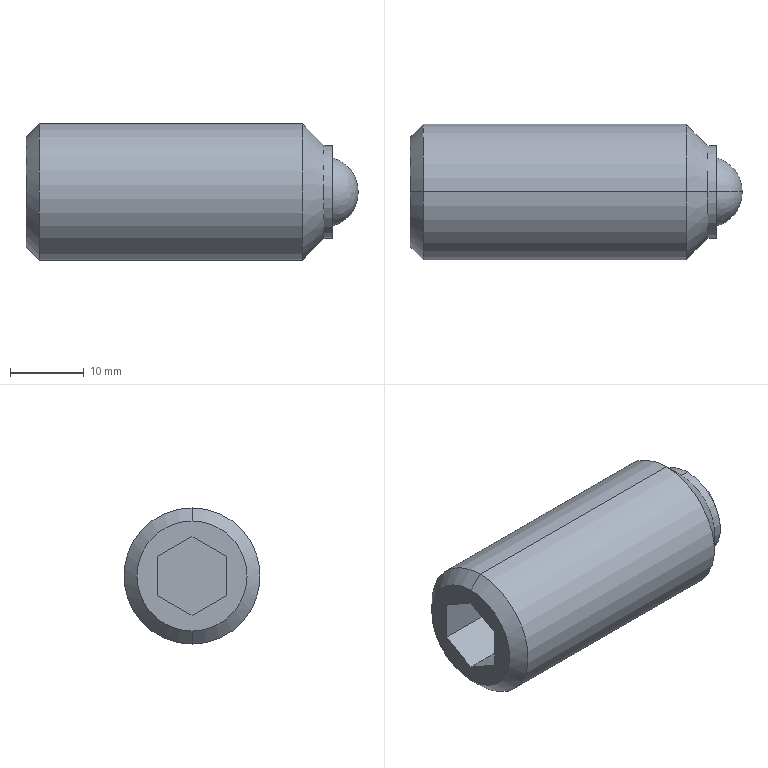Part | SolidWorks | features BaseBody 1 | 1 solid | 19 faces | box 45.002 x 18.462 x 18.462 mm | volume 10278 mm3 | plane 9 | cylinder 4 | cone 4 | spline 2 | commonest cylinder face diameters 12.614 x2 18.462 x2
STEP:
#1=CARTESIAN_POINT('',(0.09191,323.346,152.692));
#2=VERTEX_POINT('',#1);
#3=CARTESIAN_POINT('',(0.09191,323.346,134.231));
#4=VERTEX_POINT('',#3);
#5=CARTESIAN_POINT('',(0.09191,323.346,143.462));
#6=DIRECTION('',(-1.,0.,0.));
#7=DIRECTION('',(0.,0.,1.));
#8=AXIS2_PLACEMENT_3D('',#5,#6,#7);
#9=CIRCLE('',#8,9.231);
#10=EDGE_CURVE('',#2,#4,#9,.T.);
#11=ORIENTED_EDGE('',*,*,#10,.T.);
#12=CARTESIAN_POINT('',(-35.599,323.346,134.231));
#13=VERTEX_POINT('',#12);
#14=CARTESIAN_POINT('',(7.631,323.346,134.231));
#15=DIRECTION('',(-1.,0.,0.));
#16=VECTOR('',#15,1000.);
#17=LINE('',#14,#16);
#18=EDGE_CURVE('',#4,#13,#17,.T.);
#19=ORIENTED_EDGE('',*,*,#18,.T.);
#20=CARTESIAN_POINT('',(-35.599,323.346,152.692));
#21=VERTEX_POINT('',#20);
#22=CARTESIAN_POINT('',(-35.599,323.346,143.462));
#23=DIRECTION('',(1.,0.,0.));
#24=DIRECTION('',(0.,0.,1.));
#25=AXIS2_PLACEMENT_3D('',#22,#23,#24);
#26=CIRCLE('',#25,9.231);
#27=EDGE_CURVE('',#13,#21,#26,.T.);
#28=ORIENTED_EDGE('',*,*,#27,.T.);
#29=CARTESIAN_POINT('',(7.631,323.346,152.692));
#30=DIRECTION('',(-1.,0.,0.));
#31=VECTOR('',#30,1000.);
#32=LINE('',#29,#31);
#33=EDGE_CURVE('',#2,#21,#32,.T.);
#34=ORIENTED_EDGE('',*,*,#33,.F.);
#35=EDGE_LOOP('',(#11,#19,#28,#34));
#36=FACE_OUTER_BOUND('',#35,.T.);
#37=CARTESIAN_POINT('',(7.631,323.346,143.462));
#38=DIRECTION('',(-1.,0.,0.));
#39=DIRECTION('',(0.,0.,1.));
#40=AXIS2_PLACEMENT_3D('',#37,#38,#39);
#41=CYLINDRICAL_SURFACE('',#40,9.231);
#42=ADVANCED_FACE('',(#36),#41,.T.);
#43=CARTESIAN_POINT('',(-37.369,323.346,136.001));
#44=VERTEX_POINT('',#43);
#45=CARTESIAN_POINT('',(-37.369,323.346,150.922));
#46=VERTEX_POINT('',#45);
#47=CARTESIAN_POINT('',(-37.369,323.346,143.462));
#48=DIRECTION('',(1.,0.,0.));
#49=DIRECTION('',(0.,0.,-1.));
#50=AXIS2_PLACEMENT_3D('',#47,#48,#49);
#51=CIRCLE('',#50,7.461);
#52=EDGE_CURVE('',#44,#46,#51,.T.);
#53=ORIENTED_EDGE('',*,*,#52,.T.);
#54=CARTESIAN_POINT('',(-35.599,323.346,152.692));
#55=DIRECTION('',(0.7071,0.,0.7071));
#56=VECTOR('',#55,1000.);
#57=LINE('',#54,#56);
#58=EDGE_CURVE('',#46,#21,#57,.T.);
#59=ORIENTED_EDGE('',*,*,#58,.T.);
#60=ORIENTED_EDGE('',*,*,#27,.F.);
#61=CARTESIAN_POINT('',(-35.599,323.346,134.231));
#62=DIRECTION('',(0.7071,0.,-0.7071));
#63=VECTOR('',#62,1000.);
#64=LINE('',#61,#63);
#65=EDGE_CURVE('',#44,#13,#64,.T.);
#66=ORIENTED_EDGE('',*,*,#65,.F.);
#67=EDGE_LOOP('',(#53,#59,#60,#66));
#68=FACE_OUTER_BOUND('',#67,.T.);
#69=CARTESIAN_POINT('',(-35.599,323.346,143.462));
#70=DIRECTION('',(1.,0.,0.));
#71=DIRECTION('',(0.,0.,-1.));
#72=AXIS2_PLACEMENT_3D('',#69,#70,#71);
#73=CONICAL_SURFACE('',#72,9.231,0.7854);
#74=ADVANCED_FACE('',(#68),#73,.T.);
#75=CARTESIAN_POINT('',(3.016,323.346,149.768));
#76=VERTEX_POINT('',#75);
#77=CARTESIAN_POINT('',(3.016,323.346,137.155));
#78=VERTEX_POINT('',#77);
#79=CARTESIAN_POINT('',(3.016,323.346,143.462));
#80=DIRECTION('',(-1.,0.,0.));
#81=DIRECTION('',(0.,-1.,0.));
#82=AXIS2_PLACEMENT_3D('',#79,#80,#81);
#83=CIRCLE('',#82,6.307);
#84=EDGE_CURVE('',#76,#78,#83,.T.);
#85=ORIENTED_EDGE('',*,*,#84,.T.);
#86=CARTESIAN_POINT('',(0.09191,323.346,134.231));
#87=DIRECTION('',(-0.7071,0.,-0.7071));
#88=VECTOR('',#87,1000.);
#89=LINE('',#86,#88);
#90=EDGE_CURVE('',#78,#4,#89,.T.);
#91=ORIENTED_EDGE('',*,*,#90,.T.);
#92=ORIENTED_EDGE('',*,*,#10,.F.);
#93=CARTESIAN_POINT('',(0.09191,323.346,152.692));
#94=DIRECTION('',(-0.7071,0.,0.7071));
#95=VECTOR('',#94,1000.);
#96=LINE('',#93,#95);
#97=EDGE_CURVE('',#76,#2,#96,.T.);
#98=ORIENTED_EDGE('',*,*,#97,.F.);
#99=EDGE_LOOP('',(#85,#91,#92,#98));
#100=FACE_OUTER_BOUND('',#99,.T.);
#101=CARTESIAN_POINT('',(0.09191,323.346,143.462));
#102=DIRECTION('',(-1.,0.,0.));
#103=DIRECTION('',(0.,0.,1.));
#104=AXIS2_PLACEMENT_3D('',#101,#102,#103);
#105=CONICAL_SURFACE('',#104,9.231,0.7854);
#106=ADVANCED_FACE('',(#100),#105,.T.);
#107=CARTESIAN_POINT('',(4.17,323.346,149.768));
#108=VERTEX_POINT('',#107);
#109=CARTESIAN_POINT('',(4.17,323.346,137.155));
#110=VERTEX_POINT('',#109);
#111=CARTESIAN_POINT('',(4.17,323.346,143.462));
#112=DIRECTION('',(-1.,0.,0.));
#113=DIRECTION('',(0.,0.,1.));
#114=AXIS2_PLACEMENT_3D('',#111,#112,#113);
#115=CIRCLE('',#114,6.307);
#116=EDGE_CURVE('',#108,#110,#115,.T.);
#117=ORIENTED_EDGE('',*,*,#116,.T.);
#118=CARTESIAN_POINT('',(7.631,323.346,137.155));
#119=DIRECTION('',(-1.,0.,0.));
#120=VECTOR('',#119,1000.);
#121=LINE('',#118,#120);
#122=EDGE_CURVE('',#110,#78,#121,.T.);
#123=ORIENTED_EDGE('',*,*,#122,.T.);
#124=ORIENTED_EDGE('',*,*,#84,.F.);
#125=CARTESIAN_POINT('',(7.631,323.346,149.768));
#126=DIRECTION('',(-1.,0.,0.));
#127=VECTOR('',#126,1000.);
#128=LINE('',#125,#127);
#129=EDGE_CURVE('',#108,#76,#128,.T.);
#130=ORIENTED_EDGE('',*,*,#129,.F.);
#131=EDGE_LOOP('',(#117,#123,#124,#130));
#132=FACE_OUTER_BOUND('',#131,.T.);
#133=CARTESIAN_POINT('',(7.631,323.346,143.462));
#134=DIRECTION('',(-1.,0.,0.));
#135=DIRECTION('',(0.,0.,1.));
#136=AXIS2_PLACEMENT_3D('',#133,#134,#135);
#137=CYLINDRICAL_SURFACE('',#136,6.307);
#138=ADVANCED_FACE('',(#132),#137,.T.);
#139=ORIENTED_EDGE('',*,*,#18,.F.);
#140=CARTESIAN_POINT('',(0.09191,323.346,143.462));
#141=DIRECTION('',(-1.,0.,0.));
#142=DIRECTION('',(0.,0.,1.));
#143=AXIS2_PLACEMENT_3D('',#140,#141,#142);
#144=CIRCLE('',#143,9.231);
#145=EDGE_CURVE('',#4,#2,#144,.T.);
#146=ORIENTED_EDGE('',*,*,#145,.T.);
#147=ORIENTED_EDGE('',*,*,#33,.T.);
#148=CARTESIAN_POINT('',(-35.599,323.346,143.462));
#149=DIRECTION('',(1.,0.,0.));
#150=DIRECTION('',(0.,0.,1.));
#151=AXIS2_PLACEMENT_3D('',#148,#149,#150);
#152=CIRCLE('',#151,9.231);
#153=EDGE_CURVE('',#21,#13,#152,.T.);
#154=ORIENTED_EDGE('',*,*,#153,.T.);
#155=EDGE_LOOP('',(#139,#146,#147,#154));
#156=FACE_OUTER_BOUND('',#155,.T.);
#157=CARTESIAN_POINT('',(7.631,323.346,143.462));
#158=DIRECTION('',(-1.,0.,0.));
#159=DIRECTION('',(0.,0.,1.));
#160=AXIS2_PLACEMENT_3D('',#157,#158,#159);
#161=CYLINDRICAL_SURFACE('',#160,9.231);
#162=ADVANCED_FACE('',(#156),#161,.T.);
#163=ORIENTED_EDGE('',*,*,#58,.F.);
#164=CARTESIAN_POINT('',(-37.369,323.346,143.462));
#165=DIRECTION('',(1.,0.,0.));
#166=DIRECTION('',(0.,0.,-1.));
#167=AXIS2_PLACEMENT_3D('',#164,#165,#166);
#168=CIRCLE('',#167,7.461);
#169=EDGE_CURVE('',#46,#44,#168,.T.);
#170=ORIENTED_EDGE('',*,*,#169,.T.);
#171=ORIENTED_EDGE('',*,*,#65,.T.);
#172=ORIENTED_EDGE('',*,*,#153,.F.);
#173=EDGE_LOOP('',(#163,#170,#171,#172));
#174=FACE_OUTER_BOUND('',#173,.T.);
#175=CARTESIAN_POINT('',(-35.599,323.346,143.462));
#176=DIRECTION('',(1.,0.,0.));
#177=DIRECTION('',(0.,0.,-1.));
#178=AXIS2_PLACEMENT_3D('',#175,#176,#177);
#179=CONICAL_SURFACE('',#178,9.231,0.7854);
#180=ADVANCED_FACE('',(#174),#179,.T.);
#181=ORIENTED_EDGE('',*,*,#90,.F.);
#182=CARTESIAN_POINT('',(3.016,323.346,143.462));
#183=DIRECTION('',(-1.,0.,0.));
#184=DIRECTION('',(0.,-1.,0.));
#185=AXIS2_PLACEMENT_3D('',#182,#183,#184);
#186=CIRCLE('',#185,6.307);
#187=EDGE_CURVE('',#78,#76,#186,.T.);
#188=ORIENTED_EDGE('',*,*,#187,.T.);
#189=ORIENTED_EDGE('',*,*,#97,.T.);
#190=ORIENTED_EDGE('',*,*,#145,.F.);
#191=EDGE_LOOP('',(#181,#188,#189,#190));
#192=FACE_OUTER_BOUND('',#191,.T.);
#193=CARTESIAN_POINT('',(0.09191,323.346,143.462));
#194=DIRECTION('',(-1.,0.,0.));
#195=DIRECTION('',(0.,0.,1.));
#196=AXIS2_PLACEMENT_3D('',#193,#194,#195);
#197=CONICAL_SURFACE('',#196,9.231,0.7854);
#198=ADVANCED_FACE('',(#192),#197,.T.);
#199=CARTESIAN_POINT('',(-37.369,318.731,146.126));
#200=VERTEX_POINT('',#199);
#201=CARTESIAN_POINT('',(-37.369,323.346,148.791));
#202=VERTEX_POINT('',#201);
#203=CARTESIAN_POINT('',(-37.369,318.731,146.126));
#204=DIRECTION('',(0.,0.866,0.5));
#205=VECTOR('',#204,1000.);
#206=LINE('',#203,#205);
#207=EDGE_CURVE('',#200,#202,#206,.T.);
#208=ORIENTED_EDGE('',*,*,#207,.F.);
#209=CARTESIAN_POINT('',(-37.369,318.731,140.797));
#210=VERTEX_POINT('',#209);
#211=CARTESIAN_POINT('',(-37.369,318.731,143.462));
#212=DIRECTION('',(0.,0.,1.));
#213=VECTOR('',#212,1000.);
#214=LINE('',#211,#213);
#215=EDGE_CURVE('',#210,#200,#214,.T.);
#216=ORIENTED_EDGE('',*,*,#215,.F.);
#217=CARTESIAN_POINT('',(-37.369,323.346,138.132));
#218=VERTEX_POINT('',#217);
#219=CARTESIAN_POINT('',(-37.369,323.346,138.132));
#220=DIRECTION('',(0.,-0.866,0.5));
#221=VECTOR('',#220,1000.);
#222=LINE('',#219,#221);
#223=EDGE_CURVE('',#218,#210,#222,.T.);
#224=ORIENTED_EDGE('',*,*,#223,.F.);
#225=CARTESIAN_POINT('',(-37.369,327.962,140.797));
#226=VERTEX_POINT('',#225);
#227=CARTESIAN_POINT('',(-37.369,327.962,140.797));
#228=DIRECTION('',(0.,-0.866,-0.5));
#229=VECTOR('',#228,1000.);
#230=LINE('',#227,#229);
#231=EDGE_CURVE('',#226,#218,#230,.T.);
#232=ORIENTED_EDGE('',*,*,#231,.F.);
#233=CARTESIAN_POINT('',(-37.369,327.962,146.126));
#234=VERTEX_POINT('',#233);
#235=CARTESIAN_POINT('',(-37.369,327.962,143.462));
#236=DIRECTION('',(0.,0.,-1.));
#237=VECTOR('',#236,1000.);
#238=LINE('',#235,#237);
#239=EDGE_CURVE('',#234,#226,#238,.T.);
#240=ORIENTED_EDGE('',*,*,#239,.F.);
#241=CARTESIAN_POINT('',(-37.369,323.346,148.791));
#242=DIRECTION('',(0.,0.866,-0.5));
#243=VECTOR('',#242,1000.);
#244=LINE('',#241,#243);
#245=EDGE_CURVE('',#202,#234,#244,.T.);
#246=ORIENTED_EDGE('',*,*,#245,.F.);
#247=EDGE_LOOP('',(#208,#216,#224,#232,#240,#246));
#248=FACE_BOUND('',#247,.T.);
#249=ORIENTED_EDGE('',*,*,#52,.F.);
#250=ORIENTED_EDGE('',*,*,#169,.F.);
#251=EDGE_LOOP('',(#249,#250));
#252=FACE_OUTER_BOUND('',#251,.T.);
#253=CARTESIAN_POINT('',(-37.369,323.346,143.462));
#254=DIRECTION('',(1.,0.,0.));
#255=DIRECTION('',(0.,0.,-1.));
#256=AXIS2_PLACEMENT_3D('',#253,#254,#255);
#257=PLANE('',#256);
#258=ADVANCED_FACE('',(#248,#252),#257,.F.);
#259=ORIENTED_EDGE('',*,*,#122,.F.);
#260=CARTESIAN_POINT('',(4.17,323.346,143.462));
#261=DIRECTION('',(-1.,0.,0.));
#262=DIRECTION('',(0.,0.,1.));
#263=AXIS2_PLACEMENT_3D('',#260,#261,#262);
#264=CIRCLE('',#263,6.307);
#265=EDGE_CURVE('',#110,#108,#264,.T.);
#266=ORIENTED_EDGE('',*,*,#265,.T.);
#267=ORIENTED_EDGE('',*,*,#129,.T.);
#268=ORIENTED_EDGE('',*,*,#187,.F.);
#269=EDGE_LOOP('',(#259,#266,#267,#268));
#270=FACE_OUTER_BOUND('',#269,.T.);
#271=CARTESIAN_POINT('',(7.631,323.346,143.462));
#272=DIRECTION('',(-1.,0.,0.));
#273=DIRECTION('',(0.,0.,1.));
#274=AXIS2_PLACEMENT_3D('',#271,#272,#273);
#275=CYLINDRICAL_SURFACE('',#274,6.307);
#276=ADVANCED_FACE('',(#270),#275,.T.);
#277=CARTESIAN_POINT('',(-30.446,327.962,146.126));
#278=VERTEX_POINT('',#277);
#279=CARTESIAN_POINT('',(-30.446,327.962,146.126));
#280=DIRECTION('',(1.,0.,0.));
#281=VECTOR('',#280,1000.);
#282=LINE('',#279,#281);
#283=EDGE_CURVE('',#234,#278,#282,.T.);
#284=ORIENTED_EDGE('',*,*,#283,.T.);
#285=CARTESIAN_POINT('',(-30.446,323.346,148.791));
#286=VERTEX_POINT('',#285);
#287=CARTESIAN_POINT('',(-30.446,327.962,146.126));
#288=DIRECTION('',(0.,-0.866,0.5));
#289=VECTOR('',#288,1000.);
#290=LINE('',#287,#289);
#291=EDGE_CURVE('',#278,#286,#290,.T.);
#292=ORIENTED_EDGE('',*,*,#291,.T.);
#293=CARTESIAN_POINT('',(-30.446,323.346,148.791));
#294=DIRECTION('',(-1.,0.,0.));
#295=VECTOR('',#294,1000.);
#296=LINE('',#293,#295);
#297=EDGE_CURVE('',#286,#202,#296,.T.);
#298=ORIENTED_EDGE('',*,*,#297,.T.);
#299=ORIENTED_EDGE('',*,*,#245,.T.);
#300=EDGE_LOOP('',(#284,#292,#298,#299));
#301=FACE_OUTER_BOUND('',#300,.T.);
#302=CARTESIAN_POINT('',(-30.446,327.962,146.126));
#303=DIRECTION('',(0.,-0.5,-0.866));
#304=DIRECTION('',(0.,0.866,-0.5));
#305=AXIS2_PLACEMENT_3D('',#302,#303,#304);
#306=PLANE('',#305);
#307=ADVANCED_FACE('',(#301),#306,.T.);
#308=ORIENTED_EDGE('',*,*,#297,.F.);
#309=CARTESIAN_POINT('',(-30.446,318.731,146.126));
#310=VERTEX_POINT('',#309);
#311=CARTESIAN_POINT('',(-30.446,323.346,148.791));
#312=DIRECTION('',(0.,-0.866,-0.5));
#313=VECTOR('',#312,1000.);
#314=LINE('',#311,#313);
#315=EDGE_CURVE('',#286,#310,#314,.T.);
#316=ORIENTED_EDGE('',*,*,#315,.T.);
#317=CARTESIAN_POINT('',(-30.446,318.731,146.126));
#318=DIRECTION('',(-1.,0.,0.));
#319=VECTOR('',#318,1000.);
#320=LINE('',#317,#319);
#321=EDGE_CURVE('',#310,#200,#320,.T.);
#322=ORIENTED_EDGE('',*,*,#321,.T.);
#323=ORIENTED_EDGE('',*,*,#207,.T.);
#324=EDGE_LOOP('',(#308,#316,#322,#323));
#325=FACE_OUTER_BOUND('',#324,.T.);
#326=CARTESIAN_POINT('',(-30.446,323.346,148.791));
#327=DIRECTION('',(0.,0.5,-0.866));
#328=DIRECTION('',(0.,0.866,0.5));
#329=AXIS2_PLACEMENT_3D('',#326,#327,#328);
#330=PLANE('',#329);
#331=ADVANCED_FACE('',(#325),#330,.T.);
#332=ORIENTED_EDGE('',*,*,#321,.F.);
#333=CARTESIAN_POINT('',(-30.446,318.731,140.797));
#334=VERTEX_POINT('',#333);
#335=CARTESIAN_POINT('',(-30.446,318.731,146.126));
#336=DIRECTION('',(0.,0.,-1.));
#337=VECTOR('',#336,1000.);
#338=LINE('',#335,#337);
#339=EDGE_CURVE('',#310,#334,#338,.T.);
#340=ORIENTED_EDGE('',*,*,#339,.T.);
#341=CARTESIAN_POINT('',(-30.446,318.731,140.797));
#342=DIRECTION('',(-1.,0.,0.));
#343=VECTOR('',#342,1000.);
#344=LINE('',#341,#343);
#345=EDGE_CURVE('',#334,#210,#344,.T.);
#346=ORIENTED_EDGE('',*,*,#345,.T.);
#347=ORIENTED_EDGE('',*,*,#215,.T.);
#348=EDGE_LOOP('',(#332,#340,#346,#347));
#349=FACE_OUTER_BOUND('',#348,.T.);
#350=CARTESIAN_POINT('',(-30.446,318.731,146.126));
#351=DIRECTION('',(0.,1.,0.));
#352=DIRECTION('',(0.,0.,1.));
#353=AXIS2_PLACEMENT_3D('',#350,#351,#352);
#354=PLANE('',#353);
#355=ADVANCED_FACE('',(#349),#354,.T.);
#356=ORIENTED_EDGE('',*,*,#345,.F.);
#357=CARTESIAN_POINT('',(-30.446,323.346,138.132));
#358=VERTEX_POINT('',#357);
#359=CARTESIAN_POINT('',(-30.446,318.731,140.797));
#360=DIRECTION('',(0.,0.866,-0.5));
#361=VECTOR('',#360,1000.);
#362=LINE('',#359,#361);
#363=EDGE_CURVE('',#334,#358,#362,.T.);
#364=ORIENTED_EDGE('',*,*,#363,.T.);
#365=CARTESIAN_POINT('',(-30.446,323.346,138.132));
#366=DIRECTION('',(-1.,0.,0.));
#367=VECTOR('',#366,1000.);
#368=LINE('',#365,#367);
#369=EDGE_CURVE('',#358,#218,#368,.T.);
#370=ORIENTED_EDGE('',*,*,#369,.T.);
#371=ORIENTED_EDGE('',*,*,#223,.T.);
#372=EDGE_LOOP('',(#356,#364,#370,#371));
#373=FACE_OUTER_BOUND('',#372,.T.);
#374=CARTESIAN_POINT('',(-30.446,318.731,140.797));
#375=DIRECTION('',(0.,0.5,0.866));
#376=DIRECTION('',(0.,-0.866,0.5));
#377=AXIS2_PLACEMENT_3D('',#374,#375,#376);
#378=PLANE('',#377);
#379=ADVANCED_FACE('',(#373),#378,.T.);
#380=ORIENTED_EDGE('',*,*,#369,.F.);
#381=CARTESIAN_POINT('',(-30.446,327.962,140.797));
#382=VERTEX_POINT('',#381);
#383=CARTESIAN_POINT('',(-30.446,323.346,138.132));
#384=DIRECTION('',(0.,0.866,0.5));
#385=VECTOR('',#384,1000.);
#386=LINE('',#383,#385);
#387=EDGE_CURVE('',#358,#382,#386,.T.);
#388=ORIENTED_EDGE('',*,*,#387,.T.);
#389=CARTESIAN_POINT('',(-30.446,327.962,140.797));
#390=DIRECTION('',(-1.,0.,0.));
#391=VECTOR('',#390,1000.);
#392=LINE('',#389,#391);
#393=EDGE_CURVE('',#382,#226,#392,.T.);
#394=ORIENTED_EDGE('',*,*,#393,.T.);
#395=ORIENTED_EDGE('',*,*,#231,.T.);
#396=EDGE_LOOP('',(#380,#388,#394,#395));
#397=FACE_OUTER_BOUND('',#396,.T.);
#398=CARTESIAN_POINT('',(-30.446,323.346,138.132));
#399=DIRECTION('',(0.,-0.5,0.866));
#400=DIRECTION('',(0.,-0.866,-0.5));
#401=AXIS2_PLACEMENT_3D('',#398,#399,#400);
#402=PLANE('',#401);
#403=ADVANCED_FACE('',(#397),#402,.T.);
#404=ORIENTED_EDGE('',*,*,#393,.F.);
#405=CARTESIAN_POINT('',(-30.446,327.962,140.797));
#406=DIRECTION('',(0.,0.,1.));
#407=VECTOR('',#406,1000.);
#408=LINE('',#405,#407);
#409=EDGE_CURVE('',#382,#278,#408,.T.);
#410=ORIENTED_EDGE('',*,*,#409,.T.);
#411=ORIENTED_EDGE('',*,*,#283,.F.);
#412=ORIENTED_EDGE('',*,*,#239,.T.);
#413=EDGE_LOOP('',(#404,#410,#411,#412));
#414=FACE_OUTER_BOUND('',#413,.T.);
#415=CARTESIAN_POINT('',(-30.446,327.962,140.797));
#416=DIRECTION('',(0.,-1.,0.));
#417=DIRECTION('',(0.,0.,-1.));
#418=AXIS2_PLACEMENT_3D('',#415,#416,#417);
#419=PLANE('',#418);
#420=ADVANCED_FACE('',(#414),#419,.T.);
#421=CARTESIAN_POINT('',(4.17,323.346,138.846));
#422=VERTEX_POINT('',#421);
#423=CARTESIAN_POINT('',(4.17,323.346,148.077));
#424=VERTEX_POINT('',#423);
#425=CARTESIAN_POINT('',(4.17,323.346,138.846));
#426=CARTESIAN_POINT('',(4.17,326.064,138.846));
#427=CARTESIAN_POINT('',(4.17,327.962,140.772));
#428=CARTESIAN_POINT('',(4.17,327.962,143.462));
#429=CARTESIAN_POINT('',(4.17,327.962,146.151));
#430=CARTESIAN_POINT('',(4.17,326.064,148.077));
#431=CARTESIAN_POINT('',(4.17,323.346,148.077));
#432=(BOUNDED_CURVE()B_SPLINE_CURVE(3,(#425,#426,#427,#428,#429,#430,#431),.UNSPECIFIED.,.F.,.F.)B_SPLINE_CURVE_WITH_KNOTS((4,3,4),(0.,0.007213,0.01443),.UNSPECIFIED.)CURVE()GEOMETRIC_REPRESENTATION_ITEM()RATIONAL_B_SPLINE_CURVE((1.293,1.049,1.06,1.327,1.06,1.049,1.293))REPRESENTATION_ITEM(''));
#433=EDGE_CURVE('',#422,#424,#432,.T.);
#434=ORIENTED_EDGE('',*,*,#433,.F.);
#435=CARTESIAN_POINT('',(4.17,323.346,148.077));
#436=CARTESIAN_POINT('',(4.17,320.628,148.077));
#437=CARTESIAN_POINT('',(4.17,318.731,146.151));
#438=CARTESIAN_POINT('',(4.17,318.731,143.462));
#439=CARTESIAN_POINT('',(4.17,318.731,140.772));
#440=CARTESIAN_POINT('',(4.17,320.628,138.846));
#441=CARTESIAN_POINT('',(4.17,323.346,138.846));
#442=(BOUNDED_CURVE()B_SPLINE_CURVE(3,(#435,#436,#437,#438,#439,#440,#441),.UNSPECIFIED.,.F.,.F.)B_SPLINE_CURVE_WITH_KNOTS((4,3,4),(0.,0.007213,0.01443),.UNSPECIFIED.)CURVE()GEOMETRIC_REPRESENTATION_ITEM()RATIONAL_B_SPLINE_CURVE((1.293,1.049,1.06,1.327,1.06,1.049,1.293))REPRESENTATION_ITEM(''));
#443=EDGE_CURVE('',#424,#422,#442,.T.);
#444=ORIENTED_EDGE('',*,*,#443,.F.);
#445=EDGE_LOOP('',(#434,#444));
#446=FACE_BOUND('',#445,.T.);
#447=ORIENTED_EDGE('',*,*,#116,.F.);
#448=ORIENTED_EDGE('',*,*,#265,.F.);
#449=EDGE_LOOP('',(#447,#448));
#450=FACE_OUTER_BOUND('',#449,.T.);
#451=CARTESIAN_POINT('',(4.17,323.346,137.155));
#452=DIRECTION('',(-1.,0.,0.));
#453=DIRECTION('',(0.,0.,1.));
#454=AXIS2_PLACEMENT_3D('',#451,#452,#453);
#455=PLANE('',#454);
#456=ADVANCED_FACE('',(#446,#450),#455,.F.);
#457=ORIENTED_EDGE('',*,*,#315,.F.);
#458=ORIENTED_EDGE('',*,*,#291,.F.);
#459=ORIENTED_EDGE('',*,*,#409,.F.);
#460=ORIENTED_EDGE('',*,*,#387,.F.);
#461=ORIENTED_EDGE('',*,*,#363,.F.);
#462=ORIENTED_EDGE('',*,*,#339,.F.);
#463=EDGE_LOOP('',(#457,#458,#459,#460,#461,#462));
#464=FACE_OUTER_BOUND('',#463,.T.);
#465=CARTESIAN_POINT('',(-30.446,323.346,143.462));
#466=DIRECTION('',(1.,0.,0.));
#467=DIRECTION('',(0.,0.,-1.));
#468=AXIS2_PLACEMENT_3D('',#465,#466,#467);
#469=PLANE('',#468);
#470=ADVANCED_FACE('',(#464),#469,.F.);
#471=CARTESIAN_POINT('',(7.631,323.346,143.462));
#472=VERTEX_POINT('',#471);
#473=CARTESIAN_POINT('',(3.018,323.346,143.316));
#474=DIRECTION('',(0.,-1.,0.));
#475=DIRECTION('',(0.9995,0.,0.03163));
#476=AXIS2_PLACEMENT_3D('',#473,#474,#475);
#477=CIRCLE('',#476,4.615);
#478=EDGE_CURVE('',#422,#472,#477,.T.);
#479=ORIENTED_EDGE('',*,*,#478,.T.);
#480=CARTESIAN_POINT('',(3.018,323.346,143.608));
#481=DIRECTION('',(0.,-1.,0.));
#482=DIRECTION('',(0.9995,0.,-0.03163));
#483=AXIS2_PLACEMENT_3D('',#480,#481,#482);
#484=CIRCLE('',#483,4.615);
#485=EDGE_CURVE('',#472,#424,#484,.T.);
#486=ORIENTED_EDGE('',*,*,#485,.T.);
#487=ORIENTED_EDGE('',*,*,#443,.T.);
#488=EDGE_LOOP('',(#479,#486,#487));
#489=FACE_OUTER_BOUND('',#488,.T.);
#490=CARTESIAN_POINT('',(7.631,323.346,143.462));
#491=CARTESIAN_POINT('',(7.704,323.491,141.162));
#492=CARTESIAN_POINT('',(6.296,323.606,139.34));
#493=CARTESIAN_POINT('',(4.049,323.638,138.826));
#494=CARTESIAN_POINT('',(7.631,323.346,143.462));
#495=CARTESIAN_POINT('',(7.704,322.076,141.073));
#496=CARTESIAN_POINT('',(6.296,321.069,139.18));
#497=CARTESIAN_POINT('',(4.049,320.785,138.646));
#498=CARTESIAN_POINT('',(7.631,323.346,143.462));
#499=CARTESIAN_POINT('',(7.704,321.042,142.043));
#500=CARTESIAN_POINT('',(6.296,319.216,140.92));
#501=CARTESIAN_POINT('',(4.049,318.701,140.603));
#502=CARTESIAN_POINT('',(7.631,323.346,143.462));
#503=CARTESIAN_POINT('',(7.704,321.042,143.462));
#504=CARTESIAN_POINT('',(6.296,319.216,143.462));
#505=CARTESIAN_POINT('',(4.049,318.701,143.462));
#506=CARTESIAN_POINT('',(7.631,323.346,143.462));
#507=CARTESIAN_POINT('',(7.704,321.042,144.88));
#508=CARTESIAN_POINT('',(6.296,319.216,146.003));
#509=CARTESIAN_POINT('',(4.049,318.701,146.32));
#510=CARTESIAN_POINT('',(7.631,323.346,143.462));
#511=CARTESIAN_POINT('',(7.704,322.076,145.85));
#512=CARTESIAN_POINT('',(6.296,321.069,147.743));
#513=CARTESIAN_POINT('',(4.049,320.785,148.277));
#514=CARTESIAN_POINT('',(7.631,323.346,143.462));
#515=CARTESIAN_POINT('',(7.704,323.491,145.761));
#516=CARTESIAN_POINT('',(6.296,323.606,147.583));
#517=CARTESIAN_POINT('',(4.049,323.638,148.097));
#518=(BOUNDED_SURFACE()B_SPLINE_SURFACE(3,3,((#490,#491,#492,#493),(#494,#495,#496,#497),(#498,#499,#500,#501),(#502,#503,#504,#505),(#506,#507,#508,#509),(#510,#511,#512,#513),(#514,#515,#516,#517)),.UNSPECIFIED.,.F.,.F.,.F.)B_SPLINE_SURFACE_WITH_KNOTS((4,3,4),(4,4),(0.,1.,2.),(0.,1.),.UNSPECIFIED.)GEOMETRIC_REPRESENTATION_ITEM()RATIONAL_B_SPLINE_SURFACE(((1.34,1.136,1.136,1.34),(1.058,0.8974,0.8974,1.058),(1.058,0.8974,0.8974,1.058),(1.34,1.136,1.136,1.34),(1.058,0.8974,0.8974,1.058),(1.058,0.8974,0.8974,1.058),(1.34,1.136,1.136,1.34)))REPRESENTATION_ITEM('')SURFACE());
#519=ADVANCED_FACE('',(#489),#518,.T.);
#520=ORIENTED_EDGE('',*,*,#478,.F.);
#521=ORIENTED_EDGE('',*,*,#433,.T.);
#522=ORIENTED_EDGE('',*,*,#485,.F.);
#523=EDGE_LOOP('',(#520,#521,#522));
#524=FACE_OUTER_BOUND('',#523,.T.);
#525=CARTESIAN_POINT('',(7.631,323.346,143.462));
#526=CARTESIAN_POINT('',(7.704,323.202,145.761));
#527=CARTESIAN_POINT('',(6.296,323.087,147.583));
#528=CARTESIAN_POINT('',(4.049,323.055,148.097));
#529=CARTESIAN_POINT('',(7.631,323.346,143.462));
#530=CARTESIAN_POINT('',(7.704,324.617,145.85));
#531=CARTESIAN_POINT('',(6.296,325.624,147.743));
#532=CARTESIAN_POINT('',(4.049,325.907,148.277));
#533=CARTESIAN_POINT('',(7.631,323.346,143.462));
#534=CARTESIAN_POINT('',(7.704,325.651,144.88));
#535=CARTESIAN_POINT('',(6.296,327.476,146.003));
#536=CARTESIAN_POINT('',(4.049,327.991,146.32));
#537=CARTESIAN_POINT('',(7.631,323.346,143.462));
#538=CARTESIAN_POINT('',(7.704,325.651,143.462));
#539=CARTESIAN_POINT('',(6.296,327.476,143.462));
#540=CARTESIAN_POINT('',(4.049,327.991,143.462));
#541=CARTESIAN_POINT('',(7.631,323.346,143.462));
#542=CARTESIAN_POINT('',(7.704,325.651,142.043));
#543=CARTESIAN_POINT('',(6.296,327.476,140.92));
#544=CARTESIAN_POINT('',(4.049,327.991,140.603));
#545=CARTESIAN_POINT('',(7.631,323.346,143.462));
#546=CARTESIAN_POINT('',(7.704,324.617,141.073));
#547=CARTESIAN_POINT('',(6.296,325.624,139.18));
#548=CARTESIAN_POINT('',(4.049,325.907,138.646));
#549=CARTESIAN_POINT('',(7.631,323.346,143.462));
#550=CARTESIAN_POINT('',(7.704,323.202,141.162));
#551=CARTESIAN_POINT('',(6.296,323.087,139.34));
#552=CARTESIAN_POINT('',(4.049,323.055,138.826));
#553=(BOUNDED_SURFACE()B_SPLINE_SURFACE(3,3,((#525,#526,#527,#528),(#529,#530,#531,#532),(#533,#534,#535,#536),(#537,#538,#539,#540),(#541,#542,#543,#544),(#545,#546,#547,#548),(#549,#550,#551,#552)),.UNSPECIFIED.,.F.,.F.,.F.)B_SPLINE_SURFACE_WITH_KNOTS((4,3,4),(4,4),(0.,1.,2.),(0.,1.),.UNSPECIFIED.)GEOMETRIC_REPRESENTATION_ITEM()RATIONAL_B_SPLINE_SURFACE(((1.34,1.136,1.136,1.34),(1.058,0.8974,0.8974,1.058),(1.058,0.8974,0.8974,1.058),(1.34,1.136,1.136,1.34),(1.058,0.8974,0.8974,1.058),(1.058,0.8974,0.8974,1.058),(1.34,1.136,1.136,1.34)))REPRESENTATION_ITEM('')SURFACE());
#554=ADVANCED_FACE('',(#524),#553,.T.);
#555=CLOSED_SHELL('',(#42,#74,#106,#138,#162,#180,#198,#258,#276,#307,#331,#355,#379,#403,#420,#456,#470,#519,#554));
#556=MANIFOLD_SOLID_BREP('',#555);
#557=CARTESIAN_POINT('',(0.,0.,0.));
#558=DIRECTION('',(0.,0.,1.));
#559=DIRECTION('',(1.,0.,0.));
#560=AXIS2_PLACEMENT_3D('',#557,#558,#559);
#561=(LENGTH_UNIT()NAMED_UNIT(*)SI_UNIT(.MILLI.,.METRE.));
#562=UNCERTAINTY_MEASURE_WITH_UNIT(LENGTH_MEASURE(0.00001),#561,'','');
#563=(NAMED_UNIT(*)PLANE_ANGLE_UNIT()SI_UNIT($,.RADIAN.));
#564=(NAMED_UNIT(*)SI_UNIT($,.STERADIAN.)SOLID_ANGLE_UNIT());
#565=(GEOMETRIC_REPRESENTATION_CONTEXT(3)GLOBAL_UNCERTAINTY_ASSIGNED_CONTEXT((#562))GLOBAL_UNIT_ASSIGNED_CONTEXT((#561,#563,#564))REPRESENTATION_CONTEXT('',''));
#566=ADVANCED_BREP_SHAPE_REPRESENTATION('',(#556,#560),#565);